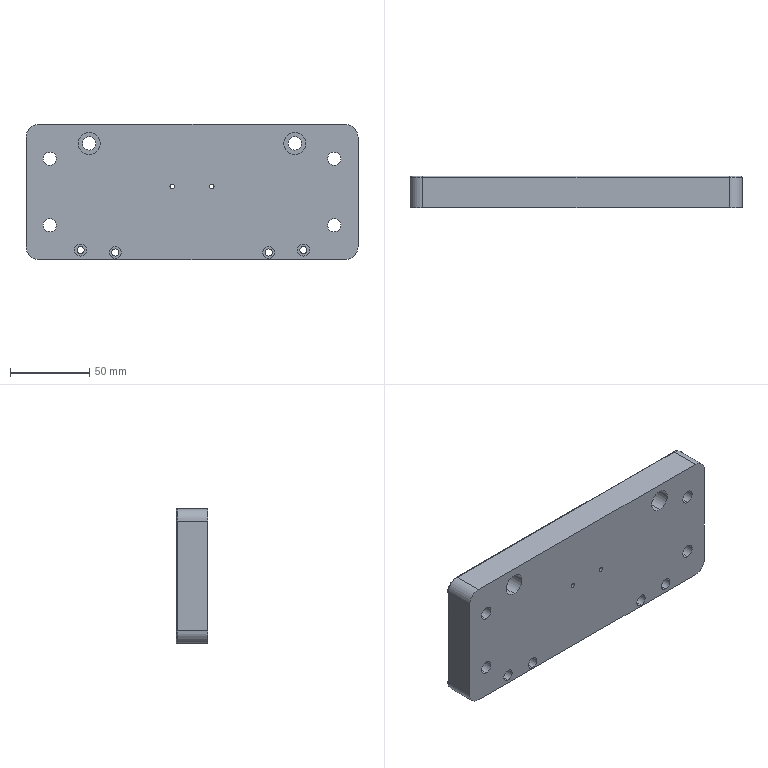Part | SolidWorks | features BaseBody 1 | 1 solid | 80 faces | box 210 x 20 x 85.5 mm | volume 334526 mm3 | cylinder 57 | plane 19 | spline 4 | commonest cylinder face diameters 8.5 x12 14 x12 4.5 x8 7.5 x8 2 x4 3 x4